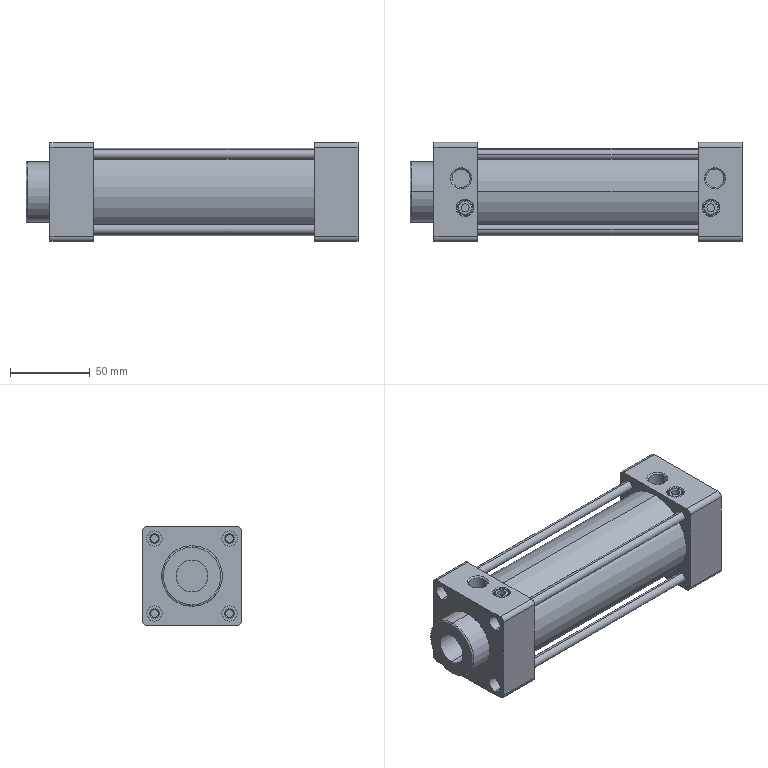Part | SolidWorks | features BaseBody 1 | 1 solid | 147 faces | box 208 x 62 x 62 mm | volume 269760 mm3 | cylinder 76 | plane 41 | cone 28 | spline 2 | commonest cylinder face diameters 4.917 x16 6 x16 9.5 x16 5 x4 9.1 x4 10.1 x4